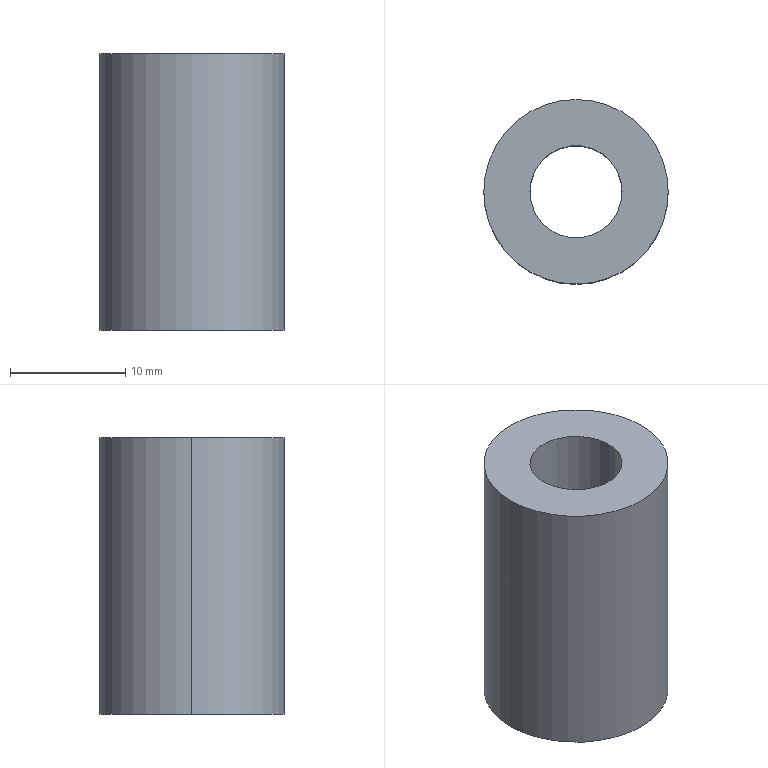Part | SolidWorks | features Extrusion 1 | 1 solid | 6 faces | box 16 x 16 x 24 mm | volume 3619 mm3 | cylinder 4 | plane 2 | commonest cylinder face diameters 8 x2 16 x2
STEP:
#1=CARTESIAN_POINT('',(-4.,0.,-12.));
#2=VERTEX_POINT('',#1);
#3=CARTESIAN_POINT('',(4.,0.,-12.));
#4=VERTEX_POINT('',#3);
#5=CARTESIAN_POINT('',(0.,0.,-12.));
#6=DIRECTION('',(0.,0.,1.));
#7=DIRECTION('',(1.,0.,0.));
#8=AXIS2_PLACEMENT_3D('',#5,#6,#7);
#9=CIRCLE('',#8,4.);
#10=EDGE_CURVE('',#2,#4,#9,.T.);
#11=ORIENTED_EDGE('',*,*,#10,.F.);
#12=CARTESIAN_POINT('',(-4.,0.,12.));
#13=VERTEX_POINT('',#12);
#14=CARTESIAN_POINT('',(-4.,0.,-12.));
#15=DIRECTION('',(0.,0.,1.));
#16=VECTOR('',#15,1000.);
#17=LINE('',#14,#16);
#18=EDGE_CURVE('',#2,#13,#17,.T.);
#19=ORIENTED_EDGE('',*,*,#18,.T.);
#20=CARTESIAN_POINT('',(4.,0.,12.));
#21=VERTEX_POINT('',#20);
#22=CARTESIAN_POINT('',(0.,0.,12.));
#23=DIRECTION('',(0.,0.,1.));
#24=DIRECTION('',(1.,0.,0.));
#25=AXIS2_PLACEMENT_3D('',#22,#23,#24);
#26=CIRCLE('',#25,4.);
#27=EDGE_CURVE('',#13,#21,#26,.T.);
#28=ORIENTED_EDGE('',*,*,#27,.T.);
#29=CARTESIAN_POINT('',(4.,0.,-12.));
#30=DIRECTION('',(0.,0.,1.));
#31=VECTOR('',#30,1000.);
#32=LINE('',#29,#31);
#33=EDGE_CURVE('',#4,#21,#32,.T.);
#34=ORIENTED_EDGE('',*,*,#33,.F.);
#35=EDGE_LOOP('',(#11,#19,#28,#34));
#36=FACE_OUTER_BOUND('',#35,.T.);
#37=CARTESIAN_POINT('',(0.,0.,-12.));
#38=DIRECTION('',(0.,0.,1.));
#39=DIRECTION('',(1.,0.,0.));
#40=AXIS2_PLACEMENT_3D('',#37,#38,#39);
#41=CYLINDRICAL_SURFACE('',#40,4.);
#42=ADVANCED_FACE('',(#36),#41,.F.);
#43=CARTESIAN_POINT('',(8.,0.,-12.));
#44=VERTEX_POINT('',#43);
#45=CARTESIAN_POINT('',(-8.,0.,-12.));
#46=VERTEX_POINT('',#45);
#47=CARTESIAN_POINT('',(0.,0.,-12.));
#48=DIRECTION('',(0.,0.,1.));
#49=DIRECTION('',(1.,0.,0.));
#50=AXIS2_PLACEMENT_3D('',#47,#48,#49);
#51=CIRCLE('',#50,8.);
#52=EDGE_CURVE('',#44,#46,#51,.T.);
#53=ORIENTED_EDGE('',*,*,#52,.T.);
#54=CARTESIAN_POINT('',(-8.,0.,12.));
#55=VERTEX_POINT('',#54);
#56=CARTESIAN_POINT('',(-8.,0.,-12.));
#57=DIRECTION('',(0.,0.,1.));
#58=VECTOR('',#57,1000.);
#59=LINE('',#56,#58);
#60=EDGE_CURVE('',#46,#55,#59,.T.);
#61=ORIENTED_EDGE('',*,*,#60,.T.);
#62=CARTESIAN_POINT('',(8.,0.,12.));
#63=VERTEX_POINT('',#62);
#64=CARTESIAN_POINT('',(0.,0.,12.));
#65=DIRECTION('',(0.,0.,1.));
#66=DIRECTION('',(1.,0.,0.));
#67=AXIS2_PLACEMENT_3D('',#64,#65,#66);
#68=CIRCLE('',#67,8.);
#69=EDGE_CURVE('',#63,#55,#68,.T.);
#70=ORIENTED_EDGE('',*,*,#69,.F.);
#71=CARTESIAN_POINT('',(8.,0.,-12.));
#72=DIRECTION('',(0.,0.,1.));
#73=VECTOR('',#72,1000.);
#74=LINE('',#71,#73);
#75=EDGE_CURVE('',#44,#63,#74,.T.);
#76=ORIENTED_EDGE('',*,*,#75,.F.);
#77=EDGE_LOOP('',(#53,#61,#70,#76));
#78=FACE_OUTER_BOUND('',#77,.T.);
#79=CARTESIAN_POINT('',(0.,0.,-12.));
#80=DIRECTION('',(0.,0.,1.));
#81=DIRECTION('',(1.,0.,0.));
#82=AXIS2_PLACEMENT_3D('',#79,#80,#81);
#83=CYLINDRICAL_SURFACE('',#82,8.);
#84=ADVANCED_FACE('',(#78),#83,.T.);
#85=ORIENTED_EDGE('',*,*,#60,.F.);
#86=CARTESIAN_POINT('',(0.,0.,-12.));
#87=DIRECTION('',(0.,0.,1.));
#88=DIRECTION('',(1.,0.,0.));
#89=AXIS2_PLACEMENT_3D('',#86,#87,#88);
#90=CIRCLE('',#89,8.);
#91=EDGE_CURVE('',#46,#44,#90,.T.);
#92=ORIENTED_EDGE('',*,*,#91,.T.);
#93=ORIENTED_EDGE('',*,*,#75,.T.);
#94=CARTESIAN_POINT('',(0.,0.,12.));
#95=DIRECTION('',(0.,0.,1.));
#96=DIRECTION('',(1.,0.,0.));
#97=AXIS2_PLACEMENT_3D('',#94,#95,#96);
#98=CIRCLE('',#97,8.);
#99=EDGE_CURVE('',#55,#63,#98,.T.);
#100=ORIENTED_EDGE('',*,*,#99,.F.);
#101=EDGE_LOOP('',(#85,#92,#93,#100));
#102=FACE_OUTER_BOUND('',#101,.T.);
#103=CARTESIAN_POINT('',(0.,0.,-12.));
#104=DIRECTION('',(0.,0.,1.));
#105=DIRECTION('',(1.,0.,0.));
#106=AXIS2_PLACEMENT_3D('',#103,#104,#105);
#107=CYLINDRICAL_SURFACE('',#106,8.);
#108=ADVANCED_FACE('',(#102),#107,.T.);
#109=CARTESIAN_POINT('',(0.,0.,-12.));
#110=DIRECTION('',(0.,0.,1.));
#111=DIRECTION('',(1.,0.,0.));
#112=AXIS2_PLACEMENT_3D('',#109,#110,#111);
#113=CIRCLE('',#112,4.);
#114=EDGE_CURVE('',#4,#2,#113,.T.);
#115=ORIENTED_EDGE('',*,*,#114,.T.);
#116=ORIENTED_EDGE('',*,*,#10,.T.);
#117=EDGE_LOOP('',(#115,#116));
#118=FACE_BOUND('',#117,.T.);
#119=ORIENTED_EDGE('',*,*,#52,.F.);
#120=ORIENTED_EDGE('',*,*,#91,.F.);
#121=EDGE_LOOP('',(#119,#120));
#122=FACE_OUTER_BOUND('',#121,.T.);
#123=CARTESIAN_POINT('',(0.,0.,-12.));
#124=DIRECTION('',(0.,0.,1.));
#125=DIRECTION('',(1.,0.,0.));
#126=AXIS2_PLACEMENT_3D('',#123,#124,#125);
#127=PLANE('',#126);
#128=ADVANCED_FACE('',(#118,#122),#127,.F.);
#129=CARTESIAN_POINT('',(0.,0.,12.));
#130=DIRECTION('',(0.,0.,1.));
#131=DIRECTION('',(1.,0.,0.));
#132=AXIS2_PLACEMENT_3D('',#129,#130,#131);
#133=CIRCLE('',#132,4.);
#134=EDGE_CURVE('',#21,#13,#133,.T.);
#135=ORIENTED_EDGE('',*,*,#134,.F.);
#136=ORIENTED_EDGE('',*,*,#27,.F.);
#137=EDGE_LOOP('',(#135,#136));
#138=FACE_BOUND('',#137,.T.);
#139=ORIENTED_EDGE('',*,*,#69,.T.);
#140=ORIENTED_EDGE('',*,*,#99,.T.);
#141=EDGE_LOOP('',(#139,#140));
#142=FACE_OUTER_BOUND('',#141,.T.);
#143=CARTESIAN_POINT('',(0.,0.,12.));
#144=DIRECTION('',(0.,0.,1.));
#145=DIRECTION('',(1.,0.,0.));
#146=AXIS2_PLACEMENT_3D('',#143,#144,#145);
#147=PLANE('',#146);
#148=ADVANCED_FACE('',(#138,#142),#147,.T.);
#149=ORIENTED_EDGE('',*,*,#18,.F.);
#150=ORIENTED_EDGE('',*,*,#114,.F.);
#151=ORIENTED_EDGE('',*,*,#33,.T.);
#152=ORIENTED_EDGE('',*,*,#134,.T.);
#153=EDGE_LOOP('',(#149,#150,#151,#152));
#154=FACE_OUTER_BOUND('',#153,.T.);
#155=CARTESIAN_POINT('',(0.,0.,-12.));
#156=DIRECTION('',(0.,0.,1.));
#157=DIRECTION('',(1.,0.,0.));
#158=AXIS2_PLACEMENT_3D('',#155,#156,#157);
#159=CYLINDRICAL_SURFACE('',#158,4.);
#160=ADVANCED_FACE('',(#154),#159,.F.);
#161=CLOSED_SHELL('',(#42,#84,#108,#128,#148,#160));
#162=MANIFOLD_SOLID_BREP('',#161);
#163=CARTESIAN_POINT('',(0.,0.,0.));
#164=DIRECTION('',(0.,0.,1.));
#165=DIRECTION('',(1.,0.,0.));
#166=AXIS2_PLACEMENT_3D('',#163,#164,#165);
#167=(LENGTH_UNIT()NAMED_UNIT(*)SI_UNIT(.MILLI.,.METRE.));
#168=UNCERTAINTY_MEASURE_WITH_UNIT(LENGTH_MEASURE(0.00001),#167,'','');
#169=(NAMED_UNIT(*)PLANE_ANGLE_UNIT()SI_UNIT($,.RADIAN.));
#170=(NAMED_UNIT(*)SI_UNIT($,.STERADIAN.)SOLID_ANGLE_UNIT());
#171=(GEOMETRIC_REPRESENTATION_CONTEXT(3)GLOBAL_UNCERTAINTY_ASSIGNED_CONTEXT((#168))GLOBAL_UNIT_ASSIGNED_CONTEXT((#167,#169,#170))REPRESENTATION_CONTEXT('',''));
#172=ADVANCED_BREP_SHAPE_REPRESENTATION('',(#162,#166),#171);